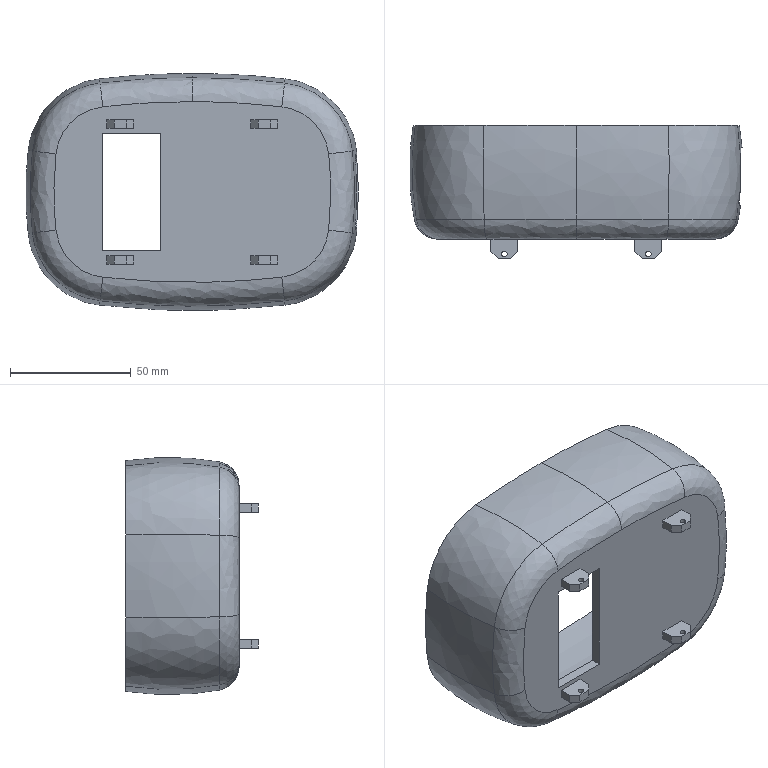Part | SolidWorks | features Cut 4, MirrorPattern 2, Chamfer 1, Extrusion 1, Fillet 1, ICE 1, Shell 1, Sweep 1 | 1 solid | 96 faces | box 137.558 x 55 x 98.119 mm | volume 101506 mm3 | plane 44 | spline 36 | cylinder 16 | commonest cylinder face diameters 2.359 x8 4 x4 8 x4